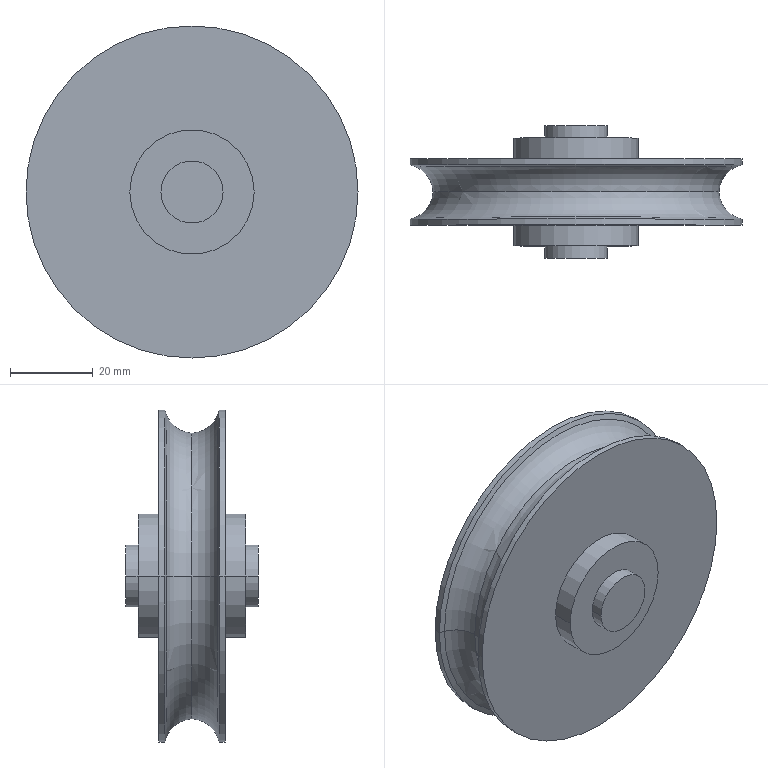Part | SolidWorks | features Revolution 1 | 1 solid | 26 faces | box 80 x 32 x 80 mm | volume 75871 mm3 | cylinder 12 | plane 6 | torus 4 | cone 4 | commonest cylinder face diameters 15 x4 30 x4 80 x4
STEP:
#1=CARTESIAN_POINT('',(-38.716,14.086,0.));
#2=VERTEX_POINT('',#1);
#3=CARTESIAN_POINT('',(-34.5,8.,0.));
#4=VERTEX_POINT('',#3);
#5=CARTESIAN_POINT('',(-41.,8.,0.));
#6=DIRECTION('',(0.,0.,-1.));
#7=DIRECTION('',(-1.,0.,0.));
#8=AXIS2_PLACEMENT_3D('',#5,#6,#7);
#9=CIRCLE('',#8,6.5);
#10=EDGE_CURVE('',#2,#4,#9,.T.);
#11=ORIENTED_EDGE('',*,*,#10,.T.);
#12=CARTESIAN_POINT('',(34.5,8.,0.));
#13=VERTEX_POINT('',#12);
#14=CARTESIAN_POINT('',(0.,8.,0.));
#15=DIRECTION('',(0.,1.,0.));
#16=DIRECTION('',(-1.,0.,0.));
#17=AXIS2_PLACEMENT_3D('',#14,#15,#16);
#18=CIRCLE('',#17,34.5);
#19=EDGE_CURVE('',#4,#13,#18,.T.);
#20=ORIENTED_EDGE('',*,*,#19,.T.);
#21=CARTESIAN_POINT('',(38.716,14.086,0.));
#22=VERTEX_POINT('',#21);
#23=CARTESIAN_POINT('',(41.,8.,0.));
#24=DIRECTION('',(0.,0.,1.));
#25=DIRECTION('',(1.,0.,0.));
#26=AXIS2_PLACEMENT_3D('',#23,#24,#25);
#27=CIRCLE('',#26,6.5);
#28=EDGE_CURVE('',#22,#13,#27,.T.);
#29=ORIENTED_EDGE('',*,*,#28,.F.);
#30=CARTESIAN_POINT('',(0.,14.086,0.));
#31=DIRECTION('',(0.,1.,0.));
#32=DIRECTION('',(-1.,0.,0.));
#33=AXIS2_PLACEMENT_3D('',#30,#31,#32);
#34=CIRCLE('',#33,38.716);
#35=EDGE_CURVE('',#2,#22,#34,.T.);
#36=ORIENTED_EDGE('',*,*,#35,.F.);
#37=EDGE_LOOP('',(#11,#20,#29,#36));
#38=FACE_OUTER_BOUND('',#37,.T.);
#39=CARTESIAN_POINT('',(0.,8.,0.));
#40=DIRECTION('',(0.,1.,0.));
#41=DIRECTION('',(-1.,0.,0.));
#42=AXIS2_PLACEMENT_3D('',#39,#40,#41);
#43=TOROIDAL_SURFACE('',#42,41.,6.5);
#44=ADVANCED_FACE('',(#38),#43,.F.);
#45=ORIENTED_EDGE('',*,*,#28,.T.);
#46=CARTESIAN_POINT('',(0.,8.,0.));
#47=DIRECTION('',(0.,1.,0.));
#48=DIRECTION('',(-1.,0.,0.));
#49=AXIS2_PLACEMENT_3D('',#46,#47,#48);
#50=CIRCLE('',#49,34.5);
#51=EDGE_CURVE('',#13,#4,#50,.T.);
#52=ORIENTED_EDGE('',*,*,#51,.T.);
#53=ORIENTED_EDGE('',*,*,#10,.F.);
#54=CARTESIAN_POINT('',(0.,14.086,0.));
#55=DIRECTION('',(0.,1.,0.));
#56=DIRECTION('',(-1.,0.,0.));
#57=AXIS2_PLACEMENT_3D('',#54,#55,#56);
#58=CIRCLE('',#57,38.716);
#59=EDGE_CURVE('',#22,#2,#58,.T.);
#60=ORIENTED_EDGE('',*,*,#59,.F.);
#61=EDGE_LOOP('',(#45,#52,#53,#60));
#62=FACE_OUTER_BOUND('',#61,.T.);
#63=CARTESIAN_POINT('',(0.,8.,0.));
#64=DIRECTION('',(0.,1.,0.));
#65=DIRECTION('',(-1.,0.,0.));
#66=AXIS2_PLACEMENT_3D('',#63,#64,#65);
#67=TOROIDAL_SURFACE('',#66,41.,6.5);
#68=ADVANCED_FACE('',(#62),#67,.F.);
#69=CARTESIAN_POINT('',(-38.716,1.914,0.));
#70=VERTEX_POINT('',#69);
#71=CARTESIAN_POINT('',(38.716,1.914,0.));
#72=VERTEX_POINT('',#71);
#73=CARTESIAN_POINT('',(0.,1.914,0.));
#74=DIRECTION('',(0.,1.,0.));
#75=DIRECTION('',(-1.,0.,0.));
#76=AXIS2_PLACEMENT_3D('',#73,#74,#75);
#77=CIRCLE('',#76,38.716);
#78=EDGE_CURVE('',#70,#72,#77,.T.);
#79=ORIENTED_EDGE('',*,*,#78,.F.);
#80=CARTESIAN_POINT('',(-40.,1.433,0.));
#81=VERTEX_POINT('',#80);
#82=CARTESIAN_POINT('',(-38.716,1.914,0.));
#83=DIRECTION('',(-0.9362,-0.3514,0.));
#84=VECTOR('',#83,1000.);
#85=LINE('',#82,#84);
#86=EDGE_CURVE('',#70,#81,#85,.T.);
#87=ORIENTED_EDGE('',*,*,#86,.T.);
#88=CARTESIAN_POINT('',(40.,1.433,0.));
#89=VERTEX_POINT('',#88);
#90=CARTESIAN_POINT('',(0.,1.433,0.));
#91=DIRECTION('',(0.,1.,0.));
#92=DIRECTION('',(-1.,0.,0.));
#93=AXIS2_PLACEMENT_3D('',#90,#91,#92);
#94=CIRCLE('',#93,40.);
#95=EDGE_CURVE('',#81,#89,#94,.T.);
#96=ORIENTED_EDGE('',*,*,#95,.T.);
#97=CARTESIAN_POINT('',(38.716,1.914,0.));
#98=DIRECTION('',(0.9362,-0.3514,0.));
#99=VECTOR('',#98,1000.);
#100=LINE('',#97,#99);
#101=EDGE_CURVE('',#72,#89,#100,.T.);
#102=ORIENTED_EDGE('',*,*,#101,.F.);
#103=EDGE_LOOP('',(#79,#87,#96,#102));
#104=FACE_OUTER_BOUND('',#103,.T.);
#105=CARTESIAN_POINT('',(0.,1.914,0.));
#106=DIRECTION('',(0.,-1.,0.));
#107=DIRECTION('',(1.,0.,0.));
#108=AXIS2_PLACEMENT_3D('',#105,#106,#107);
#109=CONICAL_SURFACE('',#108,38.716,1.212);
#110=ADVANCED_FACE('',(#104),#109,.T.);
#111=ORIENTED_EDGE('',*,*,#51,.F.);
#112=CARTESIAN_POINT('',(41.,8.,0.));
#113=DIRECTION('',(0.,0.,1.));
#114=DIRECTION('',(1.,0.,0.));
#115=AXIS2_PLACEMENT_3D('',#112,#113,#114);
#116=CIRCLE('',#115,6.5);
#117=EDGE_CURVE('',#13,#72,#116,.T.);
#118=ORIENTED_EDGE('',*,*,#117,.T.);
#119=CARTESIAN_POINT('',(0.,1.914,0.));
#120=DIRECTION('',(0.,1.,0.));
#121=DIRECTION('',(-1.,0.,0.));
#122=AXIS2_PLACEMENT_3D('',#119,#120,#121);
#123=CIRCLE('',#122,38.716);
#124=EDGE_CURVE('',#72,#70,#123,.T.);
#125=ORIENTED_EDGE('',*,*,#124,.T.);
#126=CARTESIAN_POINT('',(-41.,8.,0.));
#127=DIRECTION('',(0.,0.,-1.));
#128=DIRECTION('',(-1.,0.,0.));
#129=AXIS2_PLACEMENT_3D('',#126,#127,#128);
#130=CIRCLE('',#129,6.5);
#131=EDGE_CURVE('',#4,#70,#130,.T.);
#132=ORIENTED_EDGE('',*,*,#131,.F.);
#133=EDGE_LOOP('',(#111,#118,#125,#132));
#134=FACE_OUTER_BOUND('',#133,.T.);
#135=CARTESIAN_POINT('',(0.,8.,0.));
#136=DIRECTION('',(0.,1.,0.));
#137=DIRECTION('',(-1.,0.,0.));
#138=AXIS2_PLACEMENT_3D('',#135,#136,#137);
#139=TOROIDAL_SURFACE('',#138,41.,6.5);
#140=ADVANCED_FACE('',(#134),#139,.F.);
#141=ORIENTED_EDGE('',*,*,#35,.T.);
#142=CARTESIAN_POINT('',(40.,14.567,0.));
#143=VERTEX_POINT('',#142);
#144=CARTESIAN_POINT('',(40.,14.567,0.));
#145=DIRECTION('',(0.9362,0.3514,0.));
#146=VECTOR('',#145,1000.);
#147=LINE('',#144,#146);
#148=EDGE_CURVE('',#22,#143,#147,.T.);
#149=ORIENTED_EDGE('',*,*,#148,.T.);
#150=CARTESIAN_POINT('',(-40.,14.567,0.));
#151=VERTEX_POINT('',#150);
#152=CARTESIAN_POINT('',(0.,14.567,0.));
#153=DIRECTION('',(0.,1.,0.));
#154=DIRECTION('',(-1.,0.,0.));
#155=AXIS2_PLACEMENT_3D('',#152,#153,#154);
#156=CIRCLE('',#155,40.);
#157=EDGE_CURVE('',#151,#143,#156,.T.);
#158=ORIENTED_EDGE('',*,*,#157,.F.);
#159=CARTESIAN_POINT('',(-40.,14.567,0.));
#160=DIRECTION('',(-0.9362,0.3514,0.));
#161=VECTOR('',#160,1000.);
#162=LINE('',#159,#161);
#163=EDGE_CURVE('',#2,#151,#162,.T.);
#164=ORIENTED_EDGE('',*,*,#163,.F.);
#165=EDGE_LOOP('',(#141,#149,#158,#164));
#166=FACE_OUTER_BOUND('',#165,.T.);
#167=CARTESIAN_POINT('',(0.,14.567,0.));
#168=DIRECTION('',(0.,1.,0.));
#169=DIRECTION('',(-1.,0.,0.));
#170=AXIS2_PLACEMENT_3D('',#167,#168,#169);
#171=CONICAL_SURFACE('',#170,40.,1.212);
#172=ADVANCED_FACE('',(#166),#171,.T.);
#173=ORIENTED_EDGE('',*,*,#157,.T.);
#174=CARTESIAN_POINT('',(40.,16.,0.));
#175=VERTEX_POINT('',#174);
#176=CARTESIAN_POINT('',(40.,24.,0.));
#177=DIRECTION('',(0.,1.,0.));
#178=VECTOR('',#177,1000.);
#179=LINE('',#176,#178);
#180=EDGE_CURVE('',#143,#175,#179,.T.);
#181=ORIENTED_EDGE('',*,*,#180,.T.);
#182=CARTESIAN_POINT('',(-40.,16.,0.));
#183=VERTEX_POINT('',#182);
#184=CARTESIAN_POINT('',(0.,16.,0.));
#185=DIRECTION('',(0.,1.,0.));
#186=DIRECTION('',(-1.,0.,0.));
#187=AXIS2_PLACEMENT_3D('',#184,#185,#186);
#188=CIRCLE('',#187,40.);
#189=EDGE_CURVE('',#183,#175,#188,.T.);
#190=ORIENTED_EDGE('',*,*,#189,.F.);
#191=CARTESIAN_POINT('',(-40.,24.,0.));
#192=DIRECTION('',(0.,1.,0.));
#193=VECTOR('',#192,1000.);
#194=LINE('',#191,#193);
#195=EDGE_CURVE('',#151,#183,#194,.T.);
#196=ORIENTED_EDGE('',*,*,#195,.F.);
#197=EDGE_LOOP('',(#173,#181,#190,#196));
#198=FACE_OUTER_BOUND('',#197,.T.);
#199=CARTESIAN_POINT('',(0.,24.,0.));
#200=DIRECTION('',(0.,1.,0.));
#201=DIRECTION('',(-1.,0.,0.));
#202=AXIS2_PLACEMENT_3D('',#199,#200,#201);
#203=CYLINDRICAL_SURFACE('',#202,40.);
#204=ADVANCED_FACE('',(#198),#203,.T.);
#205=CARTESIAN_POINT('',(-15.,16.,0.));
#206=VERTEX_POINT('',#205);
#207=CARTESIAN_POINT('',(15.,16.,0.));
#208=VERTEX_POINT('',#207);
#209=CARTESIAN_POINT('',(0.,16.,0.));
#210=DIRECTION('',(0.,1.,0.));
#211=DIRECTION('',(-1.,0.,0.));
#212=AXIS2_PLACEMENT_3D('',#209,#210,#211);
#213=CIRCLE('',#212,15.);
#214=EDGE_CURVE('',#206,#208,#213,.T.);
#215=ORIENTED_EDGE('',*,*,#214,.T.);
#216=CARTESIAN_POINT('',(15.,21.,0.));
#217=VERTEX_POINT('',#216);
#218=CARTESIAN_POINT('',(15.,24.,0.));
#219=DIRECTION('',(0.,1.,0.));
#220=VECTOR('',#219,1000.);
#221=LINE('',#218,#220);
#222=EDGE_CURVE('',#208,#217,#221,.T.);
#223=ORIENTED_EDGE('',*,*,#222,.T.);
#224=CARTESIAN_POINT('',(-15.,21.,0.));
#225=VERTEX_POINT('',#224);
#226=CARTESIAN_POINT('',(0.,21.,0.));
#227=DIRECTION('',(0.,1.,0.));
#228=DIRECTION('',(-1.,0.,0.));
#229=AXIS2_PLACEMENT_3D('',#226,#227,#228);
#230=CIRCLE('',#229,15.);
#231=EDGE_CURVE('',#225,#217,#230,.T.);
#232=ORIENTED_EDGE('',*,*,#231,.F.);
#233=CARTESIAN_POINT('',(-15.,24.,0.));
#234=DIRECTION('',(0.,1.,0.));
#235=VECTOR('',#234,1000.);
#236=LINE('',#233,#235);
#237=EDGE_CURVE('',#206,#225,#236,.T.);
#238=ORIENTED_EDGE('',*,*,#237,.F.);
#239=EDGE_LOOP('',(#215,#223,#232,#238));
#240=FACE_OUTER_BOUND('',#239,.T.);
#241=CARTESIAN_POINT('',(0.,24.,0.));
#242=DIRECTION('',(0.,1.,0.));
#243=DIRECTION('',(-1.,0.,0.));
#244=AXIS2_PLACEMENT_3D('',#241,#242,#243);
#245=CYLINDRICAL_SURFACE('',#244,15.);
#246=ADVANCED_FACE('',(#240),#245,.T.);
#247=CARTESIAN_POINT('',(-7.5,21.,0.));
#248=VERTEX_POINT('',#247);
#249=CARTESIAN_POINT('',(7.5,21.,0.));
#250=VERTEX_POINT('',#249);
#251=CARTESIAN_POINT('',(0.,21.,0.));
#252=DIRECTION('',(0.,1.,0.));
#253=DIRECTION('',(-1.,0.,0.));
#254=AXIS2_PLACEMENT_3D('',#251,#252,#253);
#255=CIRCLE('',#254,7.5);
#256=EDGE_CURVE('',#248,#250,#255,.T.);
#257=ORIENTED_EDGE('',*,*,#256,.T.);
#258=CARTESIAN_POINT('',(7.5,24.,0.));
#259=VERTEX_POINT('',#258);
#260=CARTESIAN_POINT('',(7.5,24.,0.));
#261=DIRECTION('',(0.,1.,0.));
#262=VECTOR('',#261,1000.);
#263=LINE('',#260,#262);
#264=EDGE_CURVE('',#250,#259,#263,.T.);
#265=ORIENTED_EDGE('',*,*,#264,.T.);
#266=CARTESIAN_POINT('',(-7.5,24.,0.));
#267=VERTEX_POINT('',#266);
#268=CARTESIAN_POINT('',(0.,24.,0.));
#269=DIRECTION('',(0.,1.,0.));
#270=DIRECTION('',(-1.,0.,0.));
#271=AXIS2_PLACEMENT_3D('',#268,#269,#270);
#272=CIRCLE('',#271,7.5);
#273=EDGE_CURVE('',#267,#259,#272,.T.);
#274=ORIENTED_EDGE('',*,*,#273,.F.);
#275=CARTESIAN_POINT('',(-7.5,24.,0.));
#276=DIRECTION('',(0.,1.,0.));
#277=VECTOR('',#276,1000.);
#278=LINE('',#275,#277);
#279=EDGE_CURVE('',#248,#267,#278,.T.);
#280=ORIENTED_EDGE('',*,*,#279,.F.);
#281=EDGE_LOOP('',(#257,#265,#274,#280));
#282=FACE_OUTER_BOUND('',#281,.T.);
#283=CARTESIAN_POINT('',(0.,24.,0.));
#284=DIRECTION('',(0.,1.,0.));
#285=DIRECTION('',(-1.,0.,0.));
#286=AXIS2_PLACEMENT_3D('',#283,#284,#285);
#287=CYLINDRICAL_SURFACE('',#286,7.5);
#288=ADVANCED_FACE('',(#282),#287,.T.);
#289=CARTESIAN_POINT('',(-7.5,-8.,0.));
#290=VERTEX_POINT('',#289);
#291=CARTESIAN_POINT('',(7.5,-8.,0.));
#292=VERTEX_POINT('',#291);
#293=CARTESIAN_POINT('',(0.,-8.,0.));
#294=DIRECTION('',(0.,1.,0.));
#295=DIRECTION('',(-1.,0.,0.));
#296=AXIS2_PLACEMENT_3D('',#293,#294,#295);
#297=CIRCLE('',#296,7.5);
#298=EDGE_CURVE('',#290,#292,#297,.T.);
#299=ORIENTED_EDGE('',*,*,#298,.T.);
#300=CARTESIAN_POINT('',(7.5,-5.,0.));
#301=VERTEX_POINT('',#300);
#302=CARTESIAN_POINT('',(7.5,24.,0.));
#303=DIRECTION('',(0.,1.,0.));
#304=VECTOR('',#303,1000.);
#305=LINE('',#302,#304);
#306=EDGE_CURVE('',#292,#301,#305,.T.);
#307=ORIENTED_EDGE('',*,*,#306,.T.);
#308=CARTESIAN_POINT('',(-7.5,-5.,0.));
#309=VERTEX_POINT('',#308);
#310=CARTESIAN_POINT('',(0.,-5.,0.));
#311=DIRECTION('',(0.,1.,0.));
#312=DIRECTION('',(-1.,0.,0.));
#313=AXIS2_PLACEMENT_3D('',#310,#311,#312);
#314=CIRCLE('',#313,7.5);
#315=EDGE_CURVE('',#309,#301,#314,.T.);
#316=ORIENTED_EDGE('',*,*,#315,.F.);
#317=CARTESIAN_POINT('',(-7.5,24.,0.));
#318=DIRECTION('',(0.,1.,0.));
#319=VECTOR('',#318,1000.);
#320=LINE('',#317,#319);
#321=EDGE_CURVE('',#290,#309,#320,.T.);
#322=ORIENTED_EDGE('',*,*,#321,.F.);
#323=EDGE_LOOP('',(#299,#307,#316,#322));
#324=FACE_OUTER_BOUND('',#323,.T.);
#325=CARTESIAN_POINT('',(0.,24.,0.));
#326=DIRECTION('',(0.,1.,0.));
#327=DIRECTION('',(-1.,0.,0.));
#328=AXIS2_PLACEMENT_3D('',#325,#326,#327);
#329=CYLINDRICAL_SURFACE('',#328,7.5);
#330=ADVANCED_FACE('',(#324),#329,.T.);
#331=CARTESIAN_POINT('',(-15.,-5.,0.));
#332=VERTEX_POINT('',#331);
#333=CARTESIAN_POINT('',(15.,-5.,0.));
#334=VERTEX_POINT('',#333);
#335=CARTESIAN_POINT('',(0.,-5.,0.));
#336=DIRECTION('',(0.,1.,0.));
#337=DIRECTION('',(-1.,0.,0.));
#338=AXIS2_PLACEMENT_3D('',#335,#336,#337);
#339=CIRCLE('',#338,15.);
#340=EDGE_CURVE('',#332,#334,#339,.T.);
#341=ORIENTED_EDGE('',*,*,#340,.T.);
#342=CARTESIAN_POINT('',(15.,0.,0.));
#343=VERTEX_POINT('',#342);
#344=CARTESIAN_POINT('',(15.,24.,0.));
#345=DIRECTION('',(0.,1.,0.));
#346=VECTOR('',#345,1000.);
#347=LINE('',#344,#346);
#348=EDGE_CURVE('',#334,#343,#347,.T.);
#349=ORIENTED_EDGE('',*,*,#348,.T.);
#350=CARTESIAN_POINT('',(-15.,0.,0.));
#351=VERTEX_POINT('',#350);
#352=CARTESIAN_POINT('',(0.,0.,0.));
#353=DIRECTION('',(0.,1.,0.));
#354=DIRECTION('',(-1.,0.,0.));
#355=AXIS2_PLACEMENT_3D('',#352,#353,#354);
#356=CIRCLE('',#355,15.);
#357=EDGE_CURVE('',#351,#343,#356,.T.);
#358=ORIENTED_EDGE('',*,*,#357,.F.);
#359=CARTESIAN_POINT('',(-15.,24.,0.));
#360=DIRECTION('',(0.,1.,0.));
#361=VECTOR('',#360,1000.);
#362=LINE('',#359,#361);
#363=EDGE_CURVE('',#332,#351,#362,.T.);
#364=ORIENTED_EDGE('',*,*,#363,.F.);
#365=EDGE_LOOP('',(#341,#349,#358,#364));
#366=FACE_OUTER_BOUND('',#365,.T.);
#367=CARTESIAN_POINT('',(0.,24.,0.));
#368=DIRECTION('',(0.,1.,0.));
#369=DIRECTION('',(-1.,0.,0.));
#370=AXIS2_PLACEMENT_3D('',#367,#368,#369);
#371=CYLINDRICAL_SURFACE('',#370,15.);
#372=ADVANCED_FACE('',(#366),#371,.T.);
#373=CARTESIAN_POINT('',(-40.,0.,0.));
#374=VERTEX_POINT('',#373);
#375=CARTESIAN_POINT('',(40.,0.,0.));
#376=VERTEX_POINT('',#375);
#377=CARTESIAN_POINT('',(0.,0.,0.));
#378=DIRECTION('',(0.,1.,0.));
#379=DIRECTION('',(-1.,0.,0.));
#380=AXIS2_PLACEMENT_3D('',#377,#378,#379);
#381=CIRCLE('',#380,40.);
#382=EDGE_CURVE('',#374,#376,#381,.T.);
#383=ORIENTED_EDGE('',*,*,#382,.T.);
#384=CARTESIAN_POINT('',(40.,24.,0.));
#385=DIRECTION('',(0.,1.,0.));
#386=VECTOR('',#385,1000.);
#387=LINE('',#384,#386);
#388=EDGE_CURVE('',#376,#89,#387,.T.);
#389=ORIENTED_EDGE('',*,*,#388,.T.);
#390=ORIENTED_EDGE('',*,*,#95,.F.);
#391=CARTESIAN_POINT('',(-40.,24.,0.));
#392=DIRECTION('',(0.,1.,0.));
#393=VECTOR('',#392,1000.);
#394=LINE('',#391,#393);
#395=EDGE_CURVE('',#374,#81,#394,.T.);
#396=ORIENTED_EDGE('',*,*,#395,.F.);
#397=EDGE_LOOP('',(#383,#389,#390,#396));
#398=FACE_OUTER_BOUND('',#397,.T.);
#399=CARTESIAN_POINT('',(0.,24.,0.));
#400=DIRECTION('',(0.,1.,0.));
#401=DIRECTION('',(-1.,0.,0.));
#402=AXIS2_PLACEMENT_3D('',#399,#400,#401);
#403=CYLINDRICAL_SURFACE('',#402,40.);
#404=ADVANCED_FACE('',(#398),#403,.T.);
#405=ORIENTED_EDGE('',*,*,#388,.F.);
#406=CARTESIAN_POINT('',(0.,0.,0.));
#407=DIRECTION('',(0.,1.,0.));
#408=DIRECTION('',(-1.,0.,0.));
#409=AXIS2_PLACEMENT_3D('',#406,#407,#408);
#410=CIRCLE('',#409,40.);
#411=EDGE_CURVE('',#376,#374,#410,.T.);
#412=ORIENTED_EDGE('',*,*,#411,.T.);
#413=ORIENTED_EDGE('',*,*,#395,.T.);
#414=CARTESIAN_POINT('',(0.,1.433,0.));
#415=DIRECTION('',(0.,1.,0.));
#416=DIRECTION('',(-1.,0.,0.));
#417=AXIS2_PLACEMENT_3D('',#414,#415,#416);
#418=CIRCLE('',#417,40.);
#419=EDGE_CURVE('',#89,#81,#418,.T.);
#420=ORIENTED_EDGE('',*,*,#419,.F.);
#421=EDGE_LOOP('',(#405,#412,#413,#420));
#422=FACE_OUTER_BOUND('',#421,.T.);
#423=CARTESIAN_POINT('',(0.,24.,0.));
#424=DIRECTION('',(0.,1.,0.));
#425=DIRECTION('',(-1.,0.,0.));
#426=AXIS2_PLACEMENT_3D('',#423,#424,#425);
#427=CYLINDRICAL_SURFACE('',#426,40.);
#428=ADVANCED_FACE('',(#422),#427,.T.);
#429=ORIENTED_EDGE('',*,*,#357,.T.);
#430=CARTESIAN_POINT('',(0.,0.,0.));
#431=DIRECTION('',(0.,1.,0.));
#432=DIRECTION('',(-1.,0.,0.));
#433=AXIS2_PLACEMENT_3D('',#430,#431,#432);
#434=CIRCLE('',#433,15.);
#435=EDGE_CURVE('',#343,#351,#434,.T.);
#436=ORIENTED_EDGE('',*,*,#435,.T.);
#437=EDGE_LOOP('',(#429,#436));
#438=FACE_BOUND('',#437,.T.);
#439=ORIENTED_EDGE('',*,*,#382,.F.);
#440=ORIENTED_EDGE('',*,*,#411,.F.);
#441=EDGE_LOOP('',(#439,#440));
#442=FACE_OUTER_BOUND('',#441,.T.);
#443=CARTESIAN_POINT('',(-15.,0.,0.));
#444=DIRECTION('',(0.,-1.,0.));
#445=DIRECTION('',(1.,0.,0.));
#446=AXIS2_PLACEMENT_3D('',#443,#444,#445);
#447=PLANE('',#446);
#448=ADVANCED_FACE('',(#438,#442),#447,.T.);
#449=ORIENTED_EDGE('',*,*,#348,.F.);
#450=CARTESIAN_POINT('',(0.,-5.,0.));
#451=DIRECTION('',(0.,1.,0.));
#452=DIRECTION('',(-1.,0.,0.));
#453=AXIS2_PLACEMENT_3D('',#450,#451,#452);
#454=CIRCLE('',#453,15.);
#455=EDGE_CURVE('',#334,#332,#454,.T.);
#456=ORIENTED_EDGE('',*,*,#455,.T.);
#457=ORIENTED_EDGE('',*,*,#363,.T.);
#458=ORIENTED_EDGE('',*,*,#435,.F.);
#459=EDGE_LOOP('',(#449,#456,#457,#458));
#460=FACE_OUTER_BOUND('',#459,.T.);
#461=CARTESIAN_POINT('',(0.,24.,0.));
#462=DIRECTION('',(0.,1.,0.));
#463=DIRECTION('',(-1.,0.,0.));
#464=AXIS2_PLACEMENT_3D('',#461,#462,#463);
#465=CYLINDRICAL_SURFACE('',#464,15.);
#466=ADVANCED_FACE('',(#460),#465,.T.);
#467=ORIENTED_EDGE('',*,*,#315,.T.);
#468=CARTESIAN_POINT('',(0.,-5.,0.));
#469=DIRECTION('',(0.,1.,0.));
#470=DIRECTION('',(-1.,0.,0.));
#471=AXIS2_PLACEMENT_3D('',#468,#469,#470);
#472=CIRCLE('',#471,7.5);
#473=EDGE_CURVE('',#301,#309,#472,.T.);
#474=ORIENTED_EDGE('',*,*,#473,.T.);
#475=EDGE_LOOP('',(#467,#474));
#476=FACE_BOUND('',#475,.T.);
#477=ORIENTED_EDGE('',*,*,#340,.F.);
#478=ORIENTED_EDGE('',*,*,#455,.F.);
#479=EDGE_LOOP('',(#477,#478));
#480=FACE_OUTER_BOUND('',#479,.T.);
#481=CARTESIAN_POINT('',(-15.,-5.,0.));
#482=DIRECTION('',(0.,-1.,0.));
#483=DIRECTION('',(1.,0.,0.));
#484=AXIS2_PLACEMENT_3D('',#481,#482,#483);
#485=PLANE('',#484);
#486=ADVANCED_FACE('',(#476,#480),#485,.T.);
#487=ORIENTED_EDGE('',*,*,#306,.F.);
#488=CARTESIAN_POINT('',(0.,-8.,0.));
#489=DIRECTION('',(0.,1.,0.));
#490=DIRECTION('',(-1.,0.,0.));
#491=AXIS2_PLACEMENT_3D('',#488,#489,#490);
#492=CIRCLE('',#491,7.5);
#493=EDGE_CURVE('',#292,#290,#492,.T.);
#494=ORIENTED_EDGE('',*,*,#493,.T.);
#495=ORIENTED_EDGE('',*,*,#321,.T.);
#496=ORIENTED_EDGE('',*,*,#473,.F.);
#497=EDGE_LOOP('',(#487,#494,#495,#496));
#498=FACE_OUTER_BOUND('',#497,.T.);
#499=CARTESIAN_POINT('',(0.,24.,0.));
#500=DIRECTION('',(0.,1.,0.));
#501=DIRECTION('',(-1.,0.,0.));
#502=AXIS2_PLACEMENT_3D('',#499,#500,#501);
#503=CYLINDRICAL_SURFACE('',#502,7.5);
#504=ADVANCED_FACE('',(#498),#503,.T.);
#505=ORIENTED_EDGE('',*,*,#298,.F.);
#506=ORIENTED_EDGE('',*,*,#493,.F.);
#507=EDGE_LOOP('',(#505,#506));
#508=FACE_OUTER_BOUND('',#507,.T.);
#509=CARTESIAN_POINT('',(-7.5,-8.,0.));
#510=DIRECTION('',(0.,-1.,0.));
#511=DIRECTION('',(1.,0.,0.));
#512=AXIS2_PLACEMENT_3D('',#509,#510,#511);
#513=PLANE('',#512);
#514=ADVANCED_FACE('',(#508),#513,.T.);
#515=ORIENTED_EDGE('',*,*,#273,.T.);
#516=CARTESIAN_POINT('',(0.,24.,0.));
#517=DIRECTION('',(0.,1.,0.));
#518=DIRECTION('',(-1.,0.,0.));
#519=AXIS2_PLACEMENT_3D('',#516,#517,#518);
#520=CIRCLE('',#519,7.5);
#521=EDGE_CURVE('',#259,#267,#520,.T.);
#522=ORIENTED_EDGE('',*,*,#521,.T.);
#523=EDGE_LOOP('',(#515,#522));
#524=FACE_OUTER_BOUND('',#523,.T.);
#525=CARTESIAN_POINT('',(-7.5,24.,0.));
#526=DIRECTION('',(0.,1.,0.));
#527=DIRECTION('',(-1.,0.,0.));
#528=AXIS2_PLACEMENT_3D('',#525,#526,#527);
#529=PLANE('',#528);
#530=ADVANCED_FACE('',(#524),#529,.T.);
#531=ORIENTED_EDGE('',*,*,#264,.F.);
#532=CARTESIAN_POINT('',(0.,21.,0.));
#533=DIRECTION('',(0.,1.,0.));
#534=DIRECTION('',(-1.,0.,0.));
#535=AXIS2_PLACEMENT_3D('',#532,#533,#534);
#536=CIRCLE('',#535,7.5);
#537=EDGE_CURVE('',#250,#248,#536,.T.);
#538=ORIENTED_EDGE('',*,*,#537,.T.);
#539=ORIENTED_EDGE('',*,*,#279,.T.);
#540=ORIENTED_EDGE('',*,*,#521,.F.);
#541=EDGE_LOOP('',(#531,#538,#539,#540));
#542=FACE_OUTER_BOUND('',#541,.T.);
#543=CARTESIAN_POINT('',(0.,24.,0.));
#544=DIRECTION('',(0.,1.,0.));
#545=DIRECTION('',(-1.,0.,0.));
#546=AXIS2_PLACEMENT_3D('',#543,#544,#545);
#547=CYLINDRICAL_SURFACE('',#546,7.5);
#548=ADVANCED_FACE('',(#542),#547,.T.);
#549=ORIENTED_EDGE('',*,*,#231,.T.);
#550=CARTESIAN_POINT('',(0.,21.,0.));
#551=DIRECTION('',(0.,1.,0.));
#552=DIRECTION('',(-1.,0.,0.));
#553=AXIS2_PLACEMENT_3D('',#550,#551,#552);
#554=CIRCLE('',#553,15.);
#555=EDGE_CURVE('',#217,#225,#554,.T.);
#556=ORIENTED_EDGE('',*,*,#555,.T.);
#557=EDGE_LOOP('',(#549,#556));
#558=FACE_OUTER_BOUND('',#557,.T.);
#559=ORIENTED_EDGE('',*,*,#256,.F.);
#560=ORIENTED_EDGE('',*,*,#537,.F.);
#561=EDGE_LOOP('',(#559,#560));
#562=FACE_BOUND('',#561,.T.);
#563=CARTESIAN_POINT('',(-15.,21.,0.));
#564=DIRECTION('',(0.,1.,0.));
#565=DIRECTION('',(-1.,0.,0.));
#566=AXIS2_PLACEMENT_3D('',#563,#564,#565);
#567=PLANE('',#566);
#568=ADVANCED_FACE('',(#558,#562),#567,.T.);
#569=ORIENTED_EDGE('',*,*,#222,.F.);
#570=CARTESIAN_POINT('',(0.,16.,0.));
#571=DIRECTION('',(0.,1.,0.));
#572=DIRECTION('',(-1.,0.,0.));
#573=AXIS2_PLACEMENT_3D('',#570,#571,#572);
#574=CIRCLE('',#573,15.);
#575=EDGE_CURVE('',#208,#206,#574,.T.);
#576=ORIENTED_EDGE('',*,*,#575,.T.);
#577=ORIENTED_EDGE('',*,*,#237,.T.);
#578=ORIENTED_EDGE('',*,*,#555,.F.);
#579=EDGE_LOOP('',(#569,#576,#577,#578));
#580=FACE_OUTER_BOUND('',#579,.T.);
#581=CARTESIAN_POINT('',(0.,24.,0.));
#582=DIRECTION('',(0.,1.,0.));
#583=DIRECTION('',(-1.,0.,0.));
#584=AXIS2_PLACEMENT_3D('',#581,#582,#583);
#585=CYLINDRICAL_SURFACE('',#584,15.);
#586=ADVANCED_FACE('',(#580),#585,.T.);
#587=ORIENTED_EDGE('',*,*,#189,.T.);
#588=CARTESIAN_POINT('',(0.,16.,0.));
#589=DIRECTION('',(0.,1.,0.));
#590=DIRECTION('',(-1.,0.,0.));
#591=AXIS2_PLACEMENT_3D('',#588,#589,#590);
#592=CIRCLE('',#591,40.);
#593=EDGE_CURVE('',#175,#183,#592,.T.);
#594=ORIENTED_EDGE('',*,*,#593,.T.);
#595=EDGE_LOOP('',(#587,#594));
#596=FACE_OUTER_BOUND('',#595,.T.);
#597=ORIENTED_EDGE('',*,*,#214,.F.);
#598=ORIENTED_EDGE('',*,*,#575,.F.);
#599=EDGE_LOOP('',(#597,#598));
#600=FACE_BOUND('',#599,.T.);
#601=CARTESIAN_POINT('',(-40.,16.,0.));
#602=DIRECTION('',(0.,1.,0.));
#603=DIRECTION('',(-1.,0.,0.));
#604=AXIS2_PLACEMENT_3D('',#601,#602,#603);
#605=PLANE('',#604);
#606=ADVANCED_FACE('',(#596,#600),#605,.T.);
#607=ORIENTED_EDGE('',*,*,#180,.F.);
#608=CARTESIAN_POINT('',(0.,14.567,0.));
#609=DIRECTION('',(0.,1.,0.));
#610=DIRECTION('',(-1.,0.,0.));
#611=AXIS2_PLACEMENT_3D('',#608,#609,#610);
#612=CIRCLE('',#611,40.);
#613=EDGE_CURVE('',#143,#151,#612,.T.);
#614=ORIENTED_EDGE('',*,*,#613,.T.);
#615=ORIENTED_EDGE('',*,*,#195,.T.);
#616=ORIENTED_EDGE('',*,*,#593,.F.);
#617=EDGE_LOOP('',(#607,#614,#615,#616));
#618=FACE_OUTER_BOUND('',#617,.T.);
#619=CARTESIAN_POINT('',(0.,24.,0.));
#620=DIRECTION('',(0.,1.,0.));
#621=DIRECTION('',(-1.,0.,0.));
#622=AXIS2_PLACEMENT_3D('',#619,#620,#621);
#623=CYLINDRICAL_SURFACE('',#622,40.);
#624=ADVANCED_FACE('',(#618),#623,.T.);
#625=ORIENTED_EDGE('',*,*,#148,.F.);
#626=ORIENTED_EDGE('',*,*,#59,.T.);
#627=ORIENTED_EDGE('',*,*,#163,.T.);
#628=ORIENTED_EDGE('',*,*,#613,.F.);
#629=EDGE_LOOP('',(#625,#626,#627,#628));
#630=FACE_OUTER_BOUND('',#629,.T.);
#631=CARTESIAN_POINT('',(0.,14.567,0.));
#632=DIRECTION('',(0.,1.,0.));
#633=DIRECTION('',(-1.,0.,0.));
#634=AXIS2_PLACEMENT_3D('',#631,#632,#633);
#635=CONICAL_SURFACE('',#634,40.,1.212);
#636=ADVANCED_FACE('',(#630),#635,.T.);
#637=ORIENTED_EDGE('',*,*,#19,.F.);
#638=ORIENTED_EDGE('',*,*,#131,.T.);
#639=ORIENTED_EDGE('',*,*,#78,.T.);
#640=ORIENTED_EDGE('',*,*,#117,.F.);
#641=EDGE_LOOP('',(#637,#638,#639,#640));
#642=FACE_OUTER_BOUND('',#641,.T.);
#643=CARTESIAN_POINT('',(0.,8.,0.));
#644=DIRECTION('',(0.,1.,0.));
#645=DIRECTION('',(-1.,0.,0.));
#646=AXIS2_PLACEMENT_3D('',#643,#644,#645);
#647=TOROIDAL_SURFACE('',#646,41.,6.5);
#648=ADVANCED_FACE('',(#642),#647,.F.);
#649=ORIENTED_EDGE('',*,*,#86,.F.);
#650=ORIENTED_EDGE('',*,*,#124,.F.);
#651=ORIENTED_EDGE('',*,*,#101,.T.);
#652=ORIENTED_EDGE('',*,*,#419,.T.);
#653=EDGE_LOOP('',(#649,#650,#651,#652));
#654=FACE_OUTER_BOUND('',#653,.T.);
#655=CARTESIAN_POINT('',(0.,1.914,0.));
#656=DIRECTION('',(0.,-1.,0.));
#657=DIRECTION('',(1.,0.,0.));
#658=AXIS2_PLACEMENT_3D('',#655,#656,#657);
#659=CONICAL_SURFACE('',#658,38.716,1.212);
#660=ADVANCED_FACE('',(#654),#659,.T.);
#661=CLOSED_SHELL('',(#44,#68,#110,#140,#172,#204,#246,#288,#330,#372,#404,#428,#448,#466,#486,#504,#514,#530,#548,#568,#586,#606,#624,#636,#648,#660));
#662=MANIFOLD_SOLID_BREP('',#661);
#663=CARTESIAN_POINT('',(0.,0.,0.));
#664=DIRECTION('',(0.,0.,1.));
#665=DIRECTION('',(1.,0.,0.));
#666=AXIS2_PLACEMENT_3D('',#663,#664,#665);
#667=(LENGTH_UNIT()NAMED_UNIT(*)SI_UNIT(.MILLI.,.METRE.));
#668=UNCERTAINTY_MEASURE_WITH_UNIT(LENGTH_MEASURE(0.00001),#667,'','');
#669=(NAMED_UNIT(*)PLANE_ANGLE_UNIT()SI_UNIT($,.RADIAN.));
#670=(NAMED_UNIT(*)SI_UNIT($,.STERADIAN.)SOLID_ANGLE_UNIT());
#671=(GEOMETRIC_REPRESENTATION_CONTEXT(3)GLOBAL_UNCERTAINTY_ASSIGNED_CONTEXT((#668))GLOBAL_UNIT_ASSIGNED_CONTEXT((#667,#669,#670))REPRESENTATION_CONTEXT('',''));
#672=ADVANCED_BREP_SHAPE_REPRESENTATION('',(#662,#666),#671);